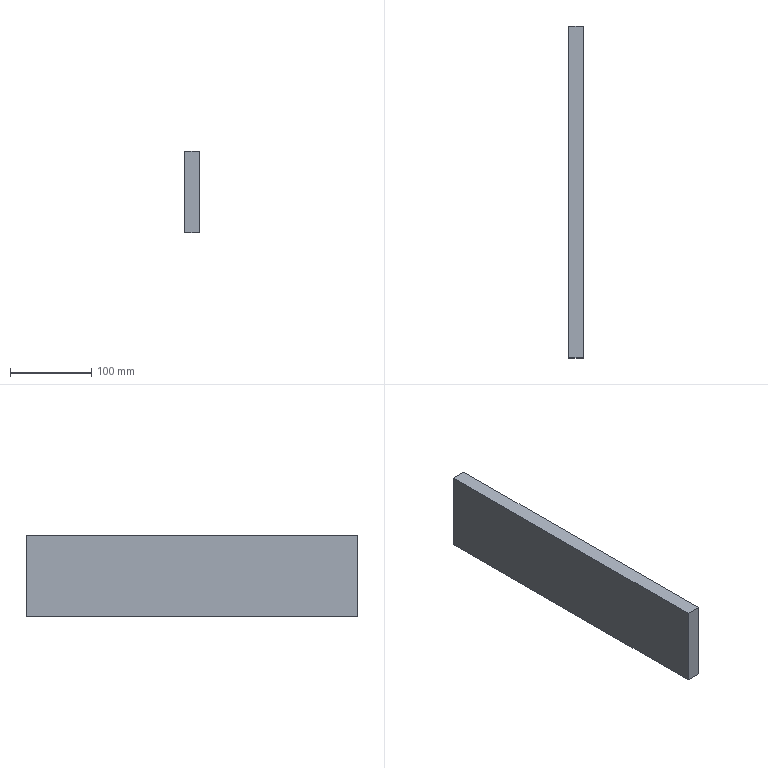Part | STEP file | Superstructure_3 | 1 solid | 6 faces | box 18 x 408 x 100 mm | volume 734400 mm3 | plane 6
STEP:
#1=CARTESIAN_POINT('',(0.,0.,0.));
#2=DIRECTION('',(0.,0.,1.));
#3=DIRECTION('',(1.,0.,0.));
#4=AXIS2_PLACEMENT_3D('',#1,#2,#3);
#5=CARTESIAN_POINT('',(-9.,204.,50.));
#6=VERTEX_POINT('',#5);
#7=CARTESIAN_POINT('',(-9.,-204.,50.));
#8=VERTEX_POINT('',#7);
#9=CARTESIAN_POINT('',(-9.,204.,50.));
#10=DIRECTION('',(0.,-1.,0.));
#11=VECTOR('',#10,1.);
#12=LINE('',#9,#11);
#13=CARTESIAN_POINT('',(-9.,204.,50.));
#14=DIRECTION('',(1.,0.,0.));
#15=DIRECTION('',(0.,0.,-1.));
#16=AXIS2_PLACEMENT_3D('',#13,#14,#15);
#17=PLANE('',#16);
#18=CARTESIAN_POINT('',(0.,0.));
#19=DIRECTION('',(0.,-1.));
#20=VECTOR('',#19,1.);
#21=LINE('',#18,#20);
#22=(GEOMETRIC_REPRESENTATION_CONTEXT(2)PARAMETRIC_REPRESENTATION_CONTEXT()REPRESENTATION_CONTEXT('',''));
#23=DEFINITIONAL_REPRESENTATION('',(#21),#22);
#24=PCURVE('',#17,#23);
#25=CARTESIAN_POINT('',(9.,204.,50.));
#26=DIRECTION('',(0.,0.,-1.));
#27=DIRECTION('',(-1.,0.,0.));
#28=AXIS2_PLACEMENT_3D('',#25,#26,#27);
#29=PLANE('',#28);
#30=CARTESIAN_POINT('',(18.,0.));
#31=DIRECTION('',(0.,-1.));
#32=VECTOR('',#31,1.);
#33=LINE('',#30,#32);
#34=(GEOMETRIC_REPRESENTATION_CONTEXT(2)PARAMETRIC_REPRESENTATION_CONTEXT()REPRESENTATION_CONTEXT('',''));
#35=DEFINITIONAL_REPRESENTATION('',(#33),#34);
#36=PCURVE('',#29,#35);
#37=SURFACE_CURVE('',#12,(#24,#36),.PCURVE_S1.);
#38=EDGE_CURVE('',#6,#8,#37,.T.);
#39=ORIENTED_EDGE('',*,*,#38,.T.);
#40=CARTESIAN_POINT('',(-9.,-204.,-50.));
#41=VERTEX_POINT('',#40);
#42=CARTESIAN_POINT('',(-9.,-204.,50.));
#43=DIRECTION('',(0.,0.,-1.));
#44=VECTOR('',#43,1.);
#45=LINE('',#42,#44);
#46=CARTESIAN_POINT('',(0.,-408.));
#47=DIRECTION('',(1.,0.));
#48=VECTOR('',#47,1.);
#49=LINE('',#46,#48);
#50=(GEOMETRIC_REPRESENTATION_CONTEXT(2)PARAMETRIC_REPRESENTATION_CONTEXT()REPRESENTATION_CONTEXT('',''));
#51=DEFINITIONAL_REPRESENTATION('',(#49),#50);
#52=PCURVE('',#17,#51);
#53=CARTESIAN_POINT('',(0.,-204.,0.));
#54=DIRECTION('',(0.,1.,0.));
#55=DIRECTION('',(0.,0.,1.));
#56=AXIS2_PLACEMENT_3D('',#53,#54,#55);
#57=PLANE('',#56);
#58=CARTESIAN_POINT('',(50.,-9.));
#59=DIRECTION('',(-1.,0.));
#60=VECTOR('',#59,1.);
#61=LINE('',#58,#60);
#62=(GEOMETRIC_REPRESENTATION_CONTEXT(2)PARAMETRIC_REPRESENTATION_CONTEXT()REPRESENTATION_CONTEXT('',''));
#63=DEFINITIONAL_REPRESENTATION('',(#61),#62);
#64=PCURVE('',#57,#63);
#65=SURFACE_CURVE('',#45,(#52,#64),.PCURVE_S1.);
#66=EDGE_CURVE('',#8,#41,#65,.T.);
#67=ORIENTED_EDGE('',*,*,#66,.T.);
#68=CARTESIAN_POINT('',(-9.,204.,-50.));
#69=VERTEX_POINT('',#68);
#70=CARTESIAN_POINT('',(-9.,204.,-50.));
#71=DIRECTION('',(0.,-1.,0.));
#72=VECTOR('',#71,1.);
#73=LINE('',#70,#72);
#74=CARTESIAN_POINT('',(100.,0.));
#75=DIRECTION('',(0.,-1.));
#76=VECTOR('',#75,1.);
#77=LINE('',#74,#76);
#78=(GEOMETRIC_REPRESENTATION_CONTEXT(2)PARAMETRIC_REPRESENTATION_CONTEXT()REPRESENTATION_CONTEXT('',''));
#79=DEFINITIONAL_REPRESENTATION('',(#77),#78);
#80=PCURVE('',#17,#79);
#81=CARTESIAN_POINT('',(-9.,204.,-50.));
#82=DIRECTION('',(0.,0.,1.));
#83=DIRECTION('',(1.,0.,0.));
#84=AXIS2_PLACEMENT_3D('',#81,#82,#83);
#85=PLANE('',#84);
#86=CARTESIAN_POINT('',(0.,0.));
#87=DIRECTION('',(0.,-1.));
#88=VECTOR('',#87,1.);
#89=LINE('',#86,#88);
#90=(GEOMETRIC_REPRESENTATION_CONTEXT(2)PARAMETRIC_REPRESENTATION_CONTEXT()REPRESENTATION_CONTEXT('',''));
#91=DEFINITIONAL_REPRESENTATION('',(#89),#90);
#92=PCURVE('',#85,#91);
#93=SURFACE_CURVE('',#73,(#80,#92),.PCURVE_S1.);
#94=EDGE_CURVE('',#69,#41,#93,.T.);
#95=ORIENTED_EDGE('',*,*,#94,.F.);
#96=CARTESIAN_POINT('',(-9.,204.,50.));
#97=DIRECTION('',(0.,0.,-1.));
#98=VECTOR('',#97,1.);
#99=LINE('',#96,#98);
#100=CARTESIAN_POINT('',(0.,0.));
#101=DIRECTION('',(1.,0.));
#102=VECTOR('',#101,1.);
#103=LINE('',#100,#102);
#104=(GEOMETRIC_REPRESENTATION_CONTEXT(2)PARAMETRIC_REPRESENTATION_CONTEXT()REPRESENTATION_CONTEXT('',''));
#105=DEFINITIONAL_REPRESENTATION('',(#103),#104);
#106=PCURVE('',#17,#105);
#107=CARTESIAN_POINT('',(0.,204.,0.));
#108=DIRECTION('',(0.,1.,0.));
#109=DIRECTION('',(0.,0.,1.));
#110=AXIS2_PLACEMENT_3D('',#107,#108,#109);
#111=PLANE('',#110);
#112=CARTESIAN_POINT('',(50.,-9.));
#113=DIRECTION('',(-1.,0.));
#114=VECTOR('',#113,1.);
#115=LINE('',#112,#114);
#116=(GEOMETRIC_REPRESENTATION_CONTEXT(2)PARAMETRIC_REPRESENTATION_CONTEXT()REPRESENTATION_CONTEXT('',''));
#117=DEFINITIONAL_REPRESENTATION('',(#115),#116);
#118=PCURVE('',#111,#117);
#119=SURFACE_CURVE('',#99,(#106,#118),.PCURVE_S1.);
#120=EDGE_CURVE('',#6,#69,#119,.T.);
#121=ORIENTED_EDGE('',*,*,#120,.F.);
#122=EDGE_LOOP('',(#39,#67,#95,#121));
#123=FACE_BOUND('',#122,.F.);
#124=ADVANCED_FACE('',(#123),#17,.F.);
#125=ORIENTED_EDGE('',*,*,#94,.T.);
#126=CARTESIAN_POINT('',(9.,-204.,-50.));
#127=VERTEX_POINT('',#126);
#128=CARTESIAN_POINT('',(-9.,-204.,-50.));
#129=DIRECTION('',(1.,0.,0.));
#130=VECTOR('',#129,1.);
#131=LINE('',#128,#130);
#132=CARTESIAN_POINT('',(0.,-408.));
#133=DIRECTION('',(1.,0.));
#134=VECTOR('',#133,1.);
#135=LINE('',#132,#134);
#136=(GEOMETRIC_REPRESENTATION_CONTEXT(2)PARAMETRIC_REPRESENTATION_CONTEXT()REPRESENTATION_CONTEXT('',''));
#137=DEFINITIONAL_REPRESENTATION('',(#135),#136);
#138=PCURVE('',#85,#137);
#139=CARTESIAN_POINT('',(-50.,-9.));
#140=DIRECTION('',(0.,1.));
#141=VECTOR('',#140,1.);
#142=LINE('',#139,#141);
#143=(GEOMETRIC_REPRESENTATION_CONTEXT(2)PARAMETRIC_REPRESENTATION_CONTEXT()REPRESENTATION_CONTEXT('',''));
#144=DEFINITIONAL_REPRESENTATION('',(#142),#143);
#145=PCURVE('',#57,#144);
#146=SURFACE_CURVE('',#131,(#138,#145),.PCURVE_S1.);
#147=EDGE_CURVE('',#41,#127,#146,.T.);
#148=ORIENTED_EDGE('',*,*,#147,.T.);
#149=CARTESIAN_POINT('',(9.,204.,-50.));
#150=VERTEX_POINT('',#149);
#151=CARTESIAN_POINT('',(9.,204.,-50.));
#152=DIRECTION('',(0.,-1.,0.));
#153=VECTOR('',#152,1.);
#154=LINE('',#151,#153);
#155=CARTESIAN_POINT('',(18.,0.));
#156=DIRECTION('',(0.,-1.));
#157=VECTOR('',#156,1.);
#158=LINE('',#155,#157);
#159=(GEOMETRIC_REPRESENTATION_CONTEXT(2)PARAMETRIC_REPRESENTATION_CONTEXT()REPRESENTATION_CONTEXT('',''));
#160=DEFINITIONAL_REPRESENTATION('',(#158),#159);
#161=PCURVE('',#85,#160);
#162=CARTESIAN_POINT('',(9.,204.,-50.));
#163=DIRECTION('',(-1.,0.,0.));
#164=DIRECTION('',(0.,0.,1.));
#165=AXIS2_PLACEMENT_3D('',#162,#163,#164);
#166=PLANE('',#165);
#167=CARTESIAN_POINT('',(0.,0.));
#168=DIRECTION('',(0.,-1.));
#169=VECTOR('',#168,1.);
#170=LINE('',#167,#169);
#171=(GEOMETRIC_REPRESENTATION_CONTEXT(2)PARAMETRIC_REPRESENTATION_CONTEXT()REPRESENTATION_CONTEXT('',''));
#172=DEFINITIONAL_REPRESENTATION('',(#170),#171);
#173=PCURVE('',#166,#172);
#174=SURFACE_CURVE('',#154,(#161,#173),.PCURVE_S1.);
#175=EDGE_CURVE('',#150,#127,#174,.T.);
#176=ORIENTED_EDGE('',*,*,#175,.F.);
#177=CARTESIAN_POINT('',(-9.,204.,-50.));
#178=DIRECTION('',(1.,0.,0.));
#179=VECTOR('',#178,1.);
#180=LINE('',#177,#179);
#181=CARTESIAN_POINT('',(0.,0.));
#182=DIRECTION('',(1.,0.));
#183=VECTOR('',#182,1.);
#184=LINE('',#181,#183);
#185=(GEOMETRIC_REPRESENTATION_CONTEXT(2)PARAMETRIC_REPRESENTATION_CONTEXT()REPRESENTATION_CONTEXT('',''));
#186=DEFINITIONAL_REPRESENTATION('',(#184),#185);
#187=PCURVE('',#85,#186);
#188=CARTESIAN_POINT('',(-50.,-9.));
#189=DIRECTION('',(0.,1.));
#190=VECTOR('',#189,1.);
#191=LINE('',#188,#190);
#192=(GEOMETRIC_REPRESENTATION_CONTEXT(2)PARAMETRIC_REPRESENTATION_CONTEXT()REPRESENTATION_CONTEXT('',''));
#193=DEFINITIONAL_REPRESENTATION('',(#191),#192);
#194=PCURVE('',#111,#193);
#195=SURFACE_CURVE('',#180,(#187,#194),.PCURVE_S1.);
#196=EDGE_CURVE('',#69,#150,#195,.T.);
#197=ORIENTED_EDGE('',*,*,#196,.F.);
#198=EDGE_LOOP('',(#125,#148,#176,#197));
#199=FACE_BOUND('',#198,.F.);
#200=ADVANCED_FACE('',(#199),#85,.F.);
#201=ORIENTED_EDGE('',*,*,#175,.T.);
#202=CARTESIAN_POINT('',(9.,-204.,50.));
#203=VERTEX_POINT('',#202);
#204=CARTESIAN_POINT('',(9.,-204.,-50.));
#205=DIRECTION('',(0.,0.,1.));
#206=VECTOR('',#205,1.);
#207=LINE('',#204,#206);
#208=CARTESIAN_POINT('',(0.,-408.));
#209=DIRECTION('',(1.,0.));
#210=VECTOR('',#209,1.);
#211=LINE('',#208,#210);
#212=(GEOMETRIC_REPRESENTATION_CONTEXT(2)PARAMETRIC_REPRESENTATION_CONTEXT()REPRESENTATION_CONTEXT('',''));
#213=DEFINITIONAL_REPRESENTATION('',(#211),#212);
#214=PCURVE('',#166,#213);
#215=CARTESIAN_POINT('',(-50.,9.));
#216=DIRECTION('',(1.,0.));
#217=VECTOR('',#216,1.);
#218=LINE('',#215,#217);
#219=(GEOMETRIC_REPRESENTATION_CONTEXT(2)PARAMETRIC_REPRESENTATION_CONTEXT()REPRESENTATION_CONTEXT('',''));
#220=DEFINITIONAL_REPRESENTATION('',(#218),#219);
#221=PCURVE('',#57,#220);
#222=SURFACE_CURVE('',#207,(#214,#221),.PCURVE_S1.);
#223=EDGE_CURVE('',#127,#203,#222,.T.);
#224=ORIENTED_EDGE('',*,*,#223,.T.);
#225=CARTESIAN_POINT('',(9.,204.,50.));
#226=VERTEX_POINT('',#225);
#227=CARTESIAN_POINT('',(9.,204.,50.));
#228=DIRECTION('',(0.,-1.,0.));
#229=VECTOR('',#228,1.);
#230=LINE('',#227,#229);
#231=CARTESIAN_POINT('',(100.,0.));
#232=DIRECTION('',(0.,-1.));
#233=VECTOR('',#232,1.);
#234=LINE('',#231,#233);
#235=(GEOMETRIC_REPRESENTATION_CONTEXT(2)PARAMETRIC_REPRESENTATION_CONTEXT()REPRESENTATION_CONTEXT('',''));
#236=DEFINITIONAL_REPRESENTATION('',(#234),#235);
#237=PCURVE('',#166,#236);
#238=CARTESIAN_POINT('',(0.,0.));
#239=DIRECTION('',(0.,-1.));
#240=VECTOR('',#239,1.);
#241=LINE('',#238,#240);
#242=(GEOMETRIC_REPRESENTATION_CONTEXT(2)PARAMETRIC_REPRESENTATION_CONTEXT()REPRESENTATION_CONTEXT('',''));
#243=DEFINITIONAL_REPRESENTATION('',(#241),#242);
#244=PCURVE('',#29,#243);
#245=SURFACE_CURVE('',#230,(#237,#244),.PCURVE_S1.);
#246=EDGE_CURVE('',#226,#203,#245,.T.);
#247=ORIENTED_EDGE('',*,*,#246,.F.);
#248=CARTESIAN_POINT('',(9.,204.,-50.));
#249=DIRECTION('',(0.,0.,1.));
#250=VECTOR('',#249,1.);
#251=LINE('',#248,#250);
#252=CARTESIAN_POINT('',(0.,0.));
#253=DIRECTION('',(1.,0.));
#254=VECTOR('',#253,1.);
#255=LINE('',#252,#254);
#256=(GEOMETRIC_REPRESENTATION_CONTEXT(2)PARAMETRIC_REPRESENTATION_CONTEXT()REPRESENTATION_CONTEXT('',''));
#257=DEFINITIONAL_REPRESENTATION('',(#255),#256);
#258=PCURVE('',#166,#257);
#259=CARTESIAN_POINT('',(-50.,9.));
#260=DIRECTION('',(1.,0.));
#261=VECTOR('',#260,1.);
#262=LINE('',#259,#261);
#263=(GEOMETRIC_REPRESENTATION_CONTEXT(2)PARAMETRIC_REPRESENTATION_CONTEXT()REPRESENTATION_CONTEXT('',''));
#264=DEFINITIONAL_REPRESENTATION('',(#262),#263);
#265=PCURVE('',#111,#264);
#266=SURFACE_CURVE('',#251,(#258,#265),.PCURVE_S1.);
#267=EDGE_CURVE('',#150,#226,#266,.T.);
#268=ORIENTED_EDGE('',*,*,#267,.F.);
#269=EDGE_LOOP('',(#201,#224,#247,#268));
#270=FACE_BOUND('',#269,.F.);
#271=ADVANCED_FACE('',(#270),#166,.F.);
#272=ORIENTED_EDGE('',*,*,#246,.T.);
#273=CARTESIAN_POINT('',(9.,-204.,50.));
#274=DIRECTION('',(-1.,0.,0.));
#275=VECTOR('',#274,1.);
#276=LINE('',#273,#275);
#277=CARTESIAN_POINT('',(0.,-408.));
#278=DIRECTION('',(1.,0.));
#279=VECTOR('',#278,1.);
#280=LINE('',#277,#279);
#281=(GEOMETRIC_REPRESENTATION_CONTEXT(2)PARAMETRIC_REPRESENTATION_CONTEXT()REPRESENTATION_CONTEXT('',''));
#282=DEFINITIONAL_REPRESENTATION('',(#280),#281);
#283=PCURVE('',#29,#282);
#284=CARTESIAN_POINT('',(50.,9.));
#285=DIRECTION('',(0.,-1.));
#286=VECTOR('',#285,1.);
#287=LINE('',#284,#286);
#288=(GEOMETRIC_REPRESENTATION_CONTEXT(2)PARAMETRIC_REPRESENTATION_CONTEXT()REPRESENTATION_CONTEXT('',''));
#289=DEFINITIONAL_REPRESENTATION('',(#287),#288);
#290=PCURVE('',#57,#289);
#291=SURFACE_CURVE('',#276,(#283,#290),.PCURVE_S1.);
#292=EDGE_CURVE('',#203,#8,#291,.T.);
#293=ORIENTED_EDGE('',*,*,#292,.T.);
#294=ORIENTED_EDGE('',*,*,#38,.F.);
#295=CARTESIAN_POINT('',(9.,204.,50.));
#296=DIRECTION('',(-1.,0.,0.));
#297=VECTOR('',#296,1.);
#298=LINE('',#295,#297);
#299=CARTESIAN_POINT('',(0.,0.));
#300=DIRECTION('',(1.,0.));
#301=VECTOR('',#300,1.);
#302=LINE('',#299,#301);
#303=(GEOMETRIC_REPRESENTATION_CONTEXT(2)PARAMETRIC_REPRESENTATION_CONTEXT()REPRESENTATION_CONTEXT('',''));
#304=DEFINITIONAL_REPRESENTATION('',(#302),#303);
#305=PCURVE('',#29,#304);
#306=CARTESIAN_POINT('',(50.,9.));
#307=DIRECTION('',(0.,-1.));
#308=VECTOR('',#307,1.);
#309=LINE('',#306,#308);
#310=(GEOMETRIC_REPRESENTATION_CONTEXT(2)PARAMETRIC_REPRESENTATION_CONTEXT()REPRESENTATION_CONTEXT('',''));
#311=DEFINITIONAL_REPRESENTATION('',(#309),#310);
#312=PCURVE('',#111,#311);
#313=SURFACE_CURVE('',#298,(#305,#312),.PCURVE_S1.);
#314=EDGE_CURVE('',#226,#6,#313,.T.);
#315=ORIENTED_EDGE('',*,*,#314,.F.);
#316=EDGE_LOOP('',(#272,#293,#294,#315));
#317=FACE_BOUND('',#316,.F.);
#318=ADVANCED_FACE('',(#317),#29,.F.);
#319=ORIENTED_EDGE('',*,*,#120,.T.);
#320=ORIENTED_EDGE('',*,*,#196,.T.);
#321=ORIENTED_EDGE('',*,*,#267,.T.);
#322=ORIENTED_EDGE('',*,*,#314,.T.);
#323=EDGE_LOOP('',(#319,#320,#321,#322));
#324=FACE_BOUND('',#323,.F.);
#325=ADVANCED_FACE('',(#324),#111,.T.);
#326=ORIENTED_EDGE('',*,*,#66,.T.);
#327=ORIENTED_EDGE('',*,*,#147,.T.);
#328=ORIENTED_EDGE('',*,*,#223,.T.);
#329=ORIENTED_EDGE('',*,*,#292,.T.);
#330=EDGE_LOOP('',(#326,#327,#328,#329));
#331=FACE_BOUND('',#330,.T.);
#332=ADVANCED_FACE('',(#331),#57,.F.);
#333=CLOSED_SHELL('',(#124,#200,#271,#318,#325,#332));
#334=MANIFOLD_SOLID_BREP('',#333);
#335=(LENGTH_UNIT()NAMED_UNIT(*)SI_UNIT(.MILLI.,.METRE.));
#336=UNCERTAINTY_MEASURE_WITH_UNIT(LENGTH_MEASURE(0.0000001),#335,'','');
#337=(NAMED_UNIT(*)PLANE_ANGLE_UNIT()SI_UNIT($,.RADIAN.));
#338=(NAMED_UNIT(*)SI_UNIT($,.STERADIAN.)SOLID_ANGLE_UNIT());
#339=(GEOMETRIC_REPRESENTATION_CONTEXT(3)GLOBAL_UNCERTAINTY_ASSIGNED_CONTEXT((#336))GLOBAL_UNIT_ASSIGNED_CONTEXT((#335,#337,#338))REPRESENTATION_CONTEXT('',''));
#340=ADVANCED_BREP_SHAPE_REPRESENTATION('',(#4,#334),#339);